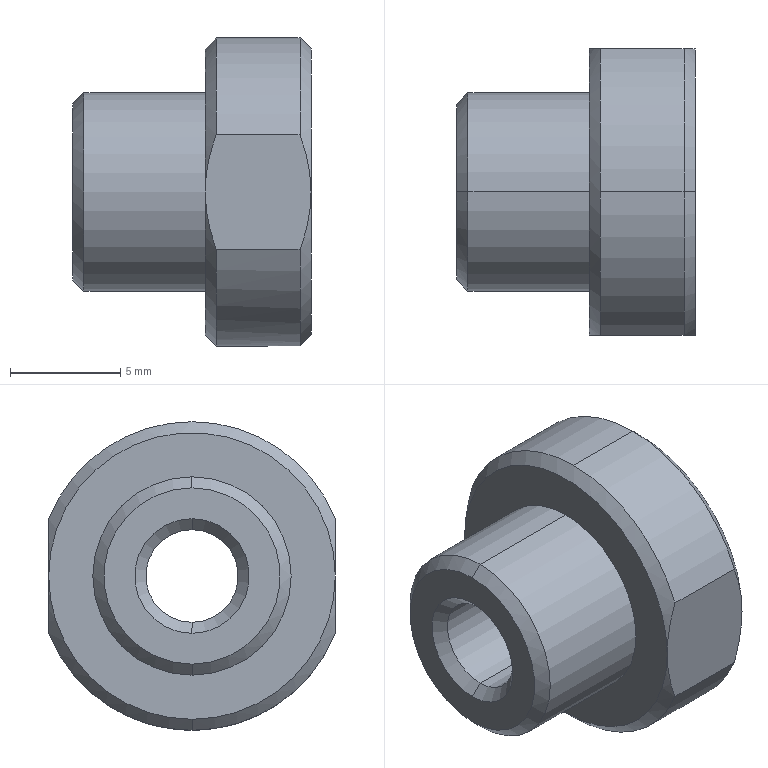Part | STEP file | PN_0070 Mount electronic clip s longitudinal manipulator movable head | 1 solid | 24 faces | box 10.8 x 13 x 14 mm | volume 938.634 mm3 | cone 12 | cylinder 7 | plane 5 | commonest cylinder face diameters 14 x3 4.2 x2 9 x2